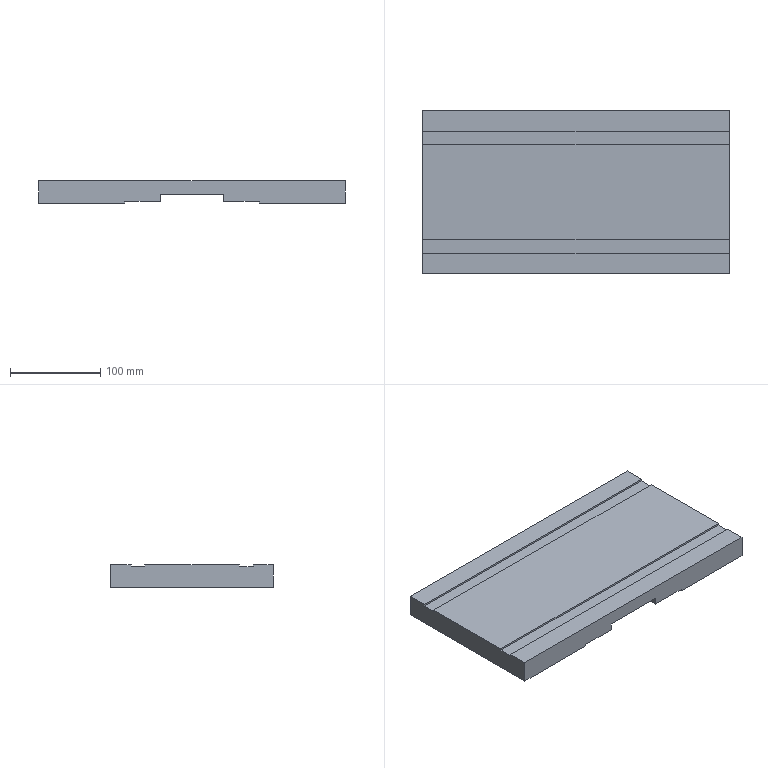Part | STEP file | 001-008-Traverse module slider connecting plate | 1 solid | 26 faces | box 340 x 180 x 25 mm | volume 1323417 mm3 | plane 24 | cylinder 2 | commonest cylinder face diameters 10 x2